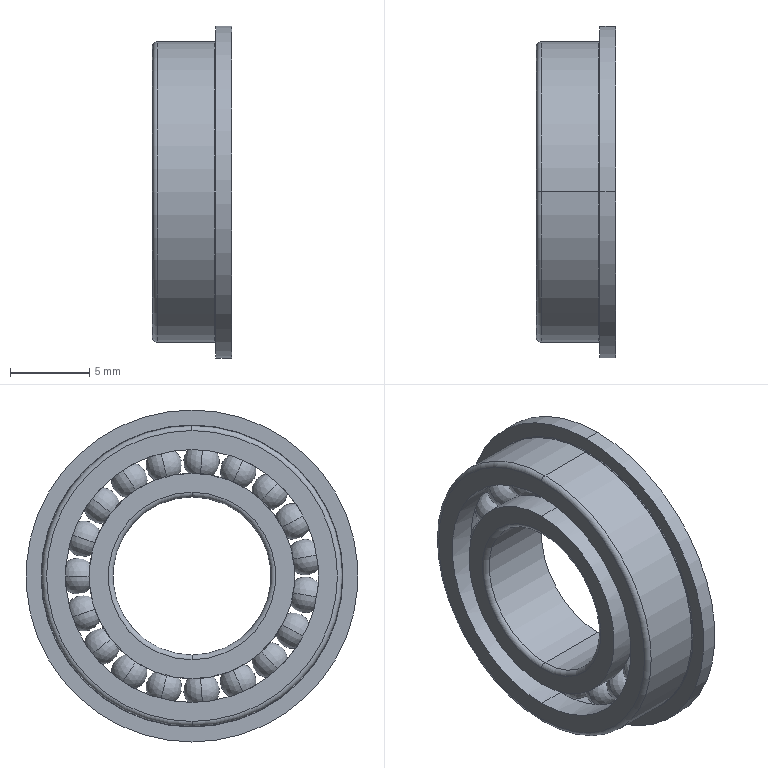Part | STEP file | miniature radial ball bearings gb_Rolling bearings FF61800  GB 7218-1995 | 1 solid | 127 faces | box 5 x 21 x 21 mm | volume 818.239 mm3 | torus 70 | sphere 38 | cylinder 14 | plane 5 | commonest cylinder face diameters 13 x4 16 x4 10 x2 19 x2 21 x2